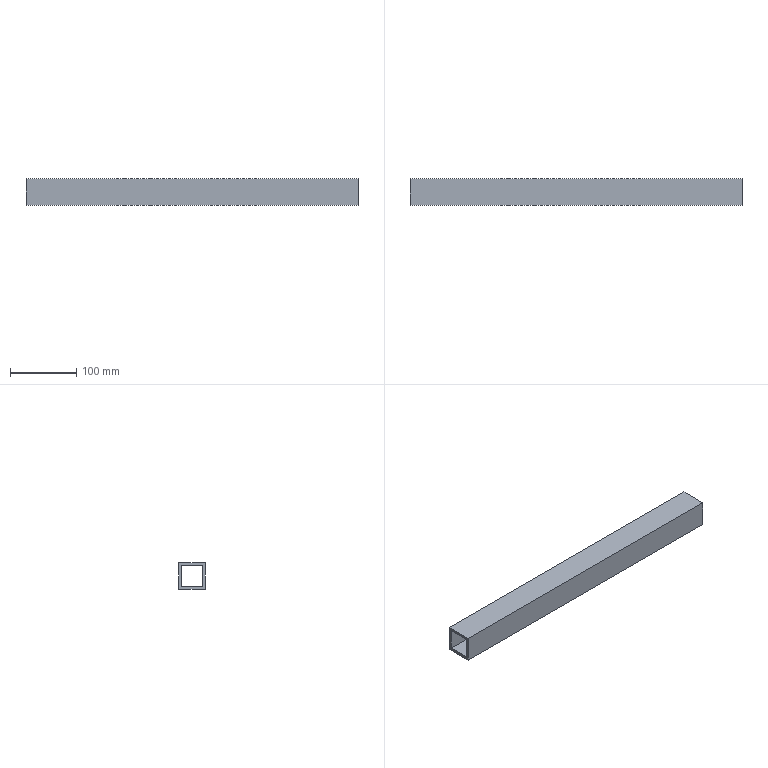Part | NX | features solid 2 | 1 solid | 10 faces | box 500 x 40 x 40 mm | volume 288000 mm3 | plane 10
STEP:
#1=CARTESIAN_POINT('',(640.,130.,-45.));
#2=VERTEX_POINT('',#1);
#3=CARTESIAN_POINT('',(1140.,130.,-45.));
#4=VERTEX_POINT('',#3);
#5=CARTESIAN_POINT('',(204.393,130.,-45.));
#6=DIRECTION('',(1.,0.,0.));
#7=VECTOR('',#6,1000.);
#8=LINE('',#5,#7);
#9=EDGE_CURVE('',#2,#4,#8,.T.);
#10=ORIENTED_EDGE('',*,*,#9,.F.);
#11=CARTESIAN_POINT('',(640.,130.,-85.));
#12=VERTEX_POINT('',#11);
#13=CARTESIAN_POINT('',(640.,130.,-70.));
#14=DIRECTION('',(0.,0.,-1.));
#15=VECTOR('',#14,1000.);
#16=LINE('',#13,#15);
#17=EDGE_CURVE('',#2,#12,#16,.T.);
#18=ORIENTED_EDGE('',*,*,#17,.T.);
#19=CARTESIAN_POINT('',(1140.,130.,-85.));
#20=VERTEX_POINT('',#19);
#21=CARTESIAN_POINT('',(119.393,130.,-85.));
#22=DIRECTION('',(1.,0.,0.));
#23=VECTOR('',#22,1000.);
#24=LINE('',#21,#23);
#25=EDGE_CURVE('',#12,#20,#24,.T.);
#26=ORIENTED_EDGE('',*,*,#25,.T.);
#27=CARTESIAN_POINT('',(1140.,130.,-70.));
#28=DIRECTION('',(0.,0.,-1.));
#29=VECTOR('',#28,1000.);
#30=LINE('',#27,#29);
#31=EDGE_CURVE('',#4,#20,#30,.T.);
#32=ORIENTED_EDGE('',*,*,#31,.F.);
#33=EDGE_LOOP('',(#10,#18,#26,#32));
#34=FACE_BOUND('',#33,.T.);
#35=CARTESIAN_POINT('',(119.393,130.,-70.));
#36=DIRECTION('',(0.,1.,0.));
#37=DIRECTION('',(0.,0.,1.));
#38=AXIS2_PLACEMENT_3D('',#35,#36,#37);
#39=PLANE('',#38);
#40=ADVANCED_FACE('',(#34),#39,.F.);
#41=ORIENTED_EDGE('',*,*,#25,.F.);
#42=CARTESIAN_POINT('',(640.,170.,-85.));
#43=VERTEX_POINT('',#42);
#44=CARTESIAN_POINT('',(640.,-450.,-85.));
#45=DIRECTION('',(0.,1.,0.));
#46=VECTOR('',#45,1000.);
#47=LINE('',#44,#46);
#48=EDGE_CURVE('',#12,#43,#47,.T.);
#49=ORIENTED_EDGE('',*,*,#48,.T.);
#50=CARTESIAN_POINT('',(1140.,170.,-85.));
#51=VERTEX_POINT('',#50);
#52=CARTESIAN_POINT('',(204.393,170.,-85.));
#53=DIRECTION('',(1.,0.,0.));
#54=VECTOR('',#53,1000.);
#55=LINE('',#52,#54);
#56=EDGE_CURVE('',#43,#51,#55,.T.);
#57=ORIENTED_EDGE('',*,*,#56,.T.);
#58=CARTESIAN_POINT('',(1140.,-450.,-85.));
#59=DIRECTION('',(0.,1.,0.));
#60=VECTOR('',#59,1000.);
#61=LINE('',#58,#60);
#62=EDGE_CURVE('',#20,#51,#61,.T.);
#63=ORIENTED_EDGE('',*,*,#62,.F.);
#64=EDGE_LOOP('',(#41,#49,#57,#63));
#65=FACE_BOUND('',#64,.T.);
#66=CARTESIAN_POINT('',(204.393,-450.,-85.));
#67=DIRECTION('',(0.,0.,1.));
#68=DIRECTION('',(0.,-1.,0.));
#69=AXIS2_PLACEMENT_3D('',#66,#67,#68);
#70=PLANE('',#69);
#71=ADVANCED_FACE('',(#65),#70,.F.);
#72=CARTESIAN_POINT('',(1140.,170.,-45.));
#73=VERTEX_POINT('',#72);
#74=CARTESIAN_POINT('',(640.,170.,-45.));
#75=VERTEX_POINT('',#74);
#76=CARTESIAN_POINT('',(204.393,170.,-45.));
#77=DIRECTION('',(-1.,0.,0.));
#78=VECTOR('',#77,1000.);
#79=LINE('',#76,#78);
#80=EDGE_CURVE('',#73,#75,#79,.T.);
#81=ORIENTED_EDGE('',*,*,#80,.T.);
#82=CARTESIAN_POINT('',(640.,-490.,-45.));
#83=DIRECTION('',(0.,-1.,0.));
#84=VECTOR('',#83,1000.);
#85=LINE('',#82,#84);
#86=EDGE_CURVE('',#75,#2,#85,.T.);
#87=ORIENTED_EDGE('',*,*,#86,.T.);
#88=ORIENTED_EDGE('',*,*,#9,.T.);
#89=CARTESIAN_POINT('',(1140.,-490.,-45.));
#90=DIRECTION('',(0.,-1.,0.));
#91=VECTOR('',#90,1000.);
#92=LINE('',#89,#91);
#93=EDGE_CURVE('',#73,#4,#92,.T.);
#94=ORIENTED_EDGE('',*,*,#93,.F.);
#95=EDGE_LOOP('',(#81,#87,#88,#94));
#96=FACE_BOUND('',#95,.T.);
#97=CARTESIAN_POINT('',(204.393,-490.,-45.));
#98=DIRECTION('',(0.,0.,-1.));
#99=DIRECTION('',(0.,1.,0.));
#100=AXIS2_PLACEMENT_3D('',#97,#98,#99);
#101=PLANE('',#100);
#102=ADVANCED_FACE('',(#96),#101,.F.);
#103=ORIENTED_EDGE('',*,*,#56,.F.);
#104=CARTESIAN_POINT('',(640.,170.,-40.));
#105=DIRECTION('',(0.,0.,1.));
#106=VECTOR('',#105,1000.);
#107=LINE('',#104,#106);
#108=EDGE_CURVE('',#43,#75,#107,.T.);
#109=ORIENTED_EDGE('',*,*,#108,.T.);
#110=ORIENTED_EDGE('',*,*,#80,.F.);
#111=CARTESIAN_POINT('',(1140.,170.,-40.));
#112=DIRECTION('',(0.,0.,1.));
#113=VECTOR('',#112,1000.);
#114=LINE('',#111,#113);
#115=EDGE_CURVE('',#51,#73,#114,.T.);
#116=ORIENTED_EDGE('',*,*,#115,.F.);
#117=EDGE_LOOP('',(#103,#109,#110,#116));
#118=FACE_BOUND('',#117,.T.);
#119=CARTESIAN_POINT('',(119.393,170.,-40.));
#120=DIRECTION('',(0.,-1.,0.));
#121=DIRECTION('',(0.,0.,-1.));
#122=AXIS2_PLACEMENT_3D('',#119,#120,#121);
#123=PLANE('',#122);
#124=ADVANCED_FACE('',(#118),#123,.F.);
#125=CARTESIAN_POINT('',(640.,134.,-49.));
#126=VERTEX_POINT('',#125);
#127=CARTESIAN_POINT('',(640.,134.,-81.));
#128=VERTEX_POINT('',#127);
#129=CARTESIAN_POINT('',(640.,134.,-70.));
#130=DIRECTION('',(0.,0.,-1.));
#131=VECTOR('',#130,1000.);
#132=LINE('',#129,#131);
#133=EDGE_CURVE('',#126,#128,#132,.T.);
#134=ORIENTED_EDGE('',*,*,#133,.F.);
#135=CARTESIAN_POINT('',(1140.,134.,-49.));
#136=VERTEX_POINT('',#135);
#137=CARTESIAN_POINT('',(204.393,134.,-49.));
#138=DIRECTION('',(1.,0.,0.));
#139=VECTOR('',#138,1000.);
#140=LINE('',#137,#139);
#141=EDGE_CURVE('',#126,#136,#140,.T.);
#142=ORIENTED_EDGE('',*,*,#141,.T.);
#143=CARTESIAN_POINT('',(1140.,134.,-81.));
#144=VERTEX_POINT('',#143);
#145=CARTESIAN_POINT('',(1140.,134.,-70.));
#146=DIRECTION('',(0.,0.,-1.));
#147=VECTOR('',#146,1000.);
#148=LINE('',#145,#147);
#149=EDGE_CURVE('',#136,#144,#148,.T.);
#150=ORIENTED_EDGE('',*,*,#149,.T.);
#151=CARTESIAN_POINT('',(119.393,134.,-81.));
#152=DIRECTION('',(1.,0.,0.));
#153=VECTOR('',#152,1000.);
#154=LINE('',#151,#153);
#155=EDGE_CURVE('',#128,#144,#154,.T.);
#156=ORIENTED_EDGE('',*,*,#155,.F.);
#157=EDGE_LOOP('',(#134,#142,#150,#156));
#158=FACE_BOUND('',#157,.T.);
#159=CARTESIAN_POINT('',(119.393,134.,-70.));
#160=DIRECTION('',(0.,1.,0.));
#161=DIRECTION('',(0.,0.,1.));
#162=AXIS2_PLACEMENT_3D('',#159,#160,#161);
#163=PLANE('',#162);
#164=ADVANCED_FACE('',(#158),#163,.T.);
#165=CARTESIAN_POINT('',(640.,166.,-81.));
#166=VERTEX_POINT('',#165);
#167=CARTESIAN_POINT('',(640.,-450.,-81.));
#168=DIRECTION('',(0.,1.,0.));
#169=VECTOR('',#168,1000.);
#170=LINE('',#167,#169);
#171=EDGE_CURVE('',#128,#166,#170,.T.);
#172=ORIENTED_EDGE('',*,*,#171,.F.);
#173=ORIENTED_EDGE('',*,*,#155,.T.);
#174=CARTESIAN_POINT('',(1140.,166.,-81.));
#175=VERTEX_POINT('',#174);
#176=CARTESIAN_POINT('',(1140.,-450.,-81.));
#177=DIRECTION('',(0.,1.,0.));
#178=VECTOR('',#177,1000.);
#179=LINE('',#176,#178);
#180=EDGE_CURVE('',#144,#175,#179,.T.);
#181=ORIENTED_EDGE('',*,*,#180,.T.);
#182=CARTESIAN_POINT('',(204.393,166.,-81.));
#183=DIRECTION('',(1.,0.,0.));
#184=VECTOR('',#183,1000.);
#185=LINE('',#182,#184);
#186=EDGE_CURVE('',#166,#175,#185,.T.);
#187=ORIENTED_EDGE('',*,*,#186,.F.);
#188=EDGE_LOOP('',(#172,#173,#181,#187));
#189=FACE_BOUND('',#188,.T.);
#190=CARTESIAN_POINT('',(204.393,-450.,-81.));
#191=DIRECTION('',(0.,0.,1.));
#192=DIRECTION('',(0.,-1.,0.));
#193=AXIS2_PLACEMENT_3D('',#190,#191,#192);
#194=PLANE('',#193);
#195=ADVANCED_FACE('',(#189),#194,.T.);
#196=CARTESIAN_POINT('',(640.,166.,-49.));
#197=VERTEX_POINT('',#196);
#198=CARTESIAN_POINT('',(640.,-490.,-49.));
#199=DIRECTION('',(0.,-1.,0.));
#200=VECTOR('',#199,1000.);
#201=LINE('',#198,#200);
#202=EDGE_CURVE('',#197,#126,#201,.T.);
#203=ORIENTED_EDGE('',*,*,#202,.F.);
#204=CARTESIAN_POINT('',(1140.,166.,-49.));
#205=VERTEX_POINT('',#204);
#206=CARTESIAN_POINT('',(204.393,166.,-49.));
#207=DIRECTION('',(-1.,0.,0.));
#208=VECTOR('',#207,1000.);
#209=LINE('',#206,#208);
#210=EDGE_CURVE('',#205,#197,#209,.T.);
#211=ORIENTED_EDGE('',*,*,#210,.F.);
#212=CARTESIAN_POINT('',(1140.,-490.,-49.));
#213=DIRECTION('',(0.,-1.,0.));
#214=VECTOR('',#213,1000.);
#215=LINE('',#212,#214);
#216=EDGE_CURVE('',#205,#136,#215,.T.);
#217=ORIENTED_EDGE('',*,*,#216,.T.);
#218=ORIENTED_EDGE('',*,*,#141,.F.);
#219=EDGE_LOOP('',(#203,#211,#217,#218));
#220=FACE_BOUND('',#219,.T.);
#221=CARTESIAN_POINT('',(204.393,-490.,-49.));
#222=DIRECTION('',(0.,0.,-1.));
#223=DIRECTION('',(0.,1.,0.));
#224=AXIS2_PLACEMENT_3D('',#221,#222,#223);
#225=PLANE('',#224);
#226=ADVANCED_FACE('',(#220),#225,.T.);
#227=CARTESIAN_POINT('',(640.,166.,-40.));
#228=DIRECTION('',(0.,0.,1.));
#229=VECTOR('',#228,1000.);
#230=LINE('',#227,#229);
#231=EDGE_CURVE('',#166,#197,#230,.T.);
#232=ORIENTED_EDGE('',*,*,#231,.F.);
#233=ORIENTED_EDGE('',*,*,#186,.T.);
#234=CARTESIAN_POINT('',(1140.,166.,-40.));
#235=DIRECTION('',(0.,0.,1.));
#236=VECTOR('',#235,1000.);
#237=LINE('',#234,#236);
#238=EDGE_CURVE('',#175,#205,#237,.T.);
#239=ORIENTED_EDGE('',*,*,#238,.T.);
#240=ORIENTED_EDGE('',*,*,#210,.T.);
#241=EDGE_LOOP('',(#232,#233,#239,#240));
#242=FACE_BOUND('',#241,.T.);
#243=CARTESIAN_POINT('',(119.393,166.,-40.));
#244=DIRECTION('',(0.,-1.,0.));
#245=DIRECTION('',(0.,0.,-1.));
#246=AXIS2_PLACEMENT_3D('',#243,#244,#245);
#247=PLANE('',#246);
#248=ADVANCED_FACE('',(#242),#247,.T.);
#249=ORIENTED_EDGE('',*,*,#149,.F.);
#250=ORIENTED_EDGE('',*,*,#216,.F.);
#251=ORIENTED_EDGE('',*,*,#238,.F.);
#252=ORIENTED_EDGE('',*,*,#180,.F.);
#253=EDGE_LOOP('',(#249,#250,#251,#252));
#254=FACE_BOUND('',#253,.T.);
#255=ORIENTED_EDGE('',*,*,#93,.T.);
#256=ORIENTED_EDGE('',*,*,#31,.T.);
#257=ORIENTED_EDGE('',*,*,#62,.T.);
#258=ORIENTED_EDGE('',*,*,#115,.T.);
#259=EDGE_LOOP('',(#255,#256,#257,#258));
#260=FACE_BOUND('',#259,.T.);
#261=CARTESIAN_POINT('',(1140.,102.5,-9.5));
#262=DIRECTION('',(1.,0.,0.));
#263=DIRECTION('',(0.,0.,-1.));
#264=AXIS2_PLACEMENT_3D('',#261,#262,#263);
#265=PLANE('',#264);
#266=ADVANCED_FACE('',(#254,#260),#265,.T.);
#267=ORIENTED_EDGE('',*,*,#133,.T.);
#268=ORIENTED_EDGE('',*,*,#171,.T.);
#269=ORIENTED_EDGE('',*,*,#231,.T.);
#270=ORIENTED_EDGE('',*,*,#202,.T.);
#271=EDGE_LOOP('',(#267,#268,#269,#270));
#272=FACE_BOUND('',#271,.T.);
#273=ORIENTED_EDGE('',*,*,#86,.F.);
#274=ORIENTED_EDGE('',*,*,#108,.F.);
#275=ORIENTED_EDGE('',*,*,#48,.F.);
#276=ORIENTED_EDGE('',*,*,#17,.F.);
#277=EDGE_LOOP('',(#273,#274,#275,#276));
#278=FACE_BOUND('',#277,.T.);
#279=CARTESIAN_POINT('',(640.,156.1,-11.));
#280=DIRECTION('',(1.,0.,0.));
#281=DIRECTION('',(0.,0.,-1.));
#282=AXIS2_PLACEMENT_3D('',#279,#280,#281);
#283=PLANE('',#282);
#284=ADVANCED_FACE('',(#272,#278),#283,.F.);
#285=CLOSED_SHELL('',(#40,#71,#102,#124,#164,#195,#226,#248,#266,#284));
#286=MANIFOLD_SOLID_BREP('',#285);
#287=(LENGTH_UNIT()NAMED_UNIT(*)SI_UNIT(.MILLI.,.METRE.));
#288=UNCERTAINTY_MEASURE_WITH_UNIT(LENGTH_MEASURE(0.00001),#287,'','');
#289=(NAMED_UNIT(*)PLANE_ANGLE_UNIT()SI_UNIT($,.RADIAN.));
#290=(NAMED_UNIT(*)SI_UNIT($,.STERADIAN.)SOLID_ANGLE_UNIT());
#291=(GEOMETRIC_REPRESENTATION_CONTEXT(3)GLOBAL_UNCERTAINTY_ASSIGNED_CONTEXT((#288))GLOBAL_UNIT_ASSIGNED_CONTEXT((#287,#289,#290))REPRESENTATION_CONTEXT('',''));
#292=ADVANCED_BREP_SHAPE_REPRESENTATION('',(#286),#291);